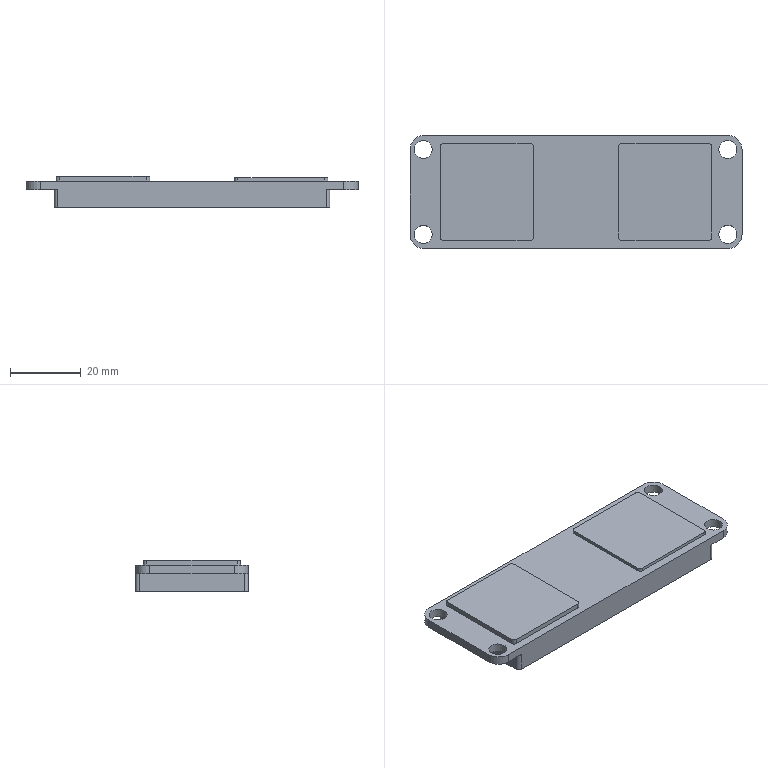CAM job | NX | 3-axis milling, drilling | part box 94 x 32 x 9 mm | stock box 94 x 32 x 9 mm
Tools:
number,name,description,diameter,corner_radius,flute_length,length,flutes
2,ER25-D10-20,Milling Tool-5 Parameters,10.0,0.0,20.0,20.0,2
3,ER25-D4-10,Milling Tool-5 Parameters,4.0,0.0,10.0,12.0,2
4,ER25-D1.5R0.3-23,Milling Tool-5 Parameters,1.5,0.3,5.0,5.0,2
10,ER25-D10-30_G,Milling Tool-5 Parameters,10.0,0.0,20.0,30.0,2
11,ER25-D4-23_G,Milling Tool-5 Parameters,4.0,0.0,10.0,23.0,2
1,D50-120,Milling Tool-5 Parameters,50.0,0.0,5.0,120.0,2
8,M3_D2.6,Drilling Tool,2.6,0.0,20.0,25.0,2
9,M3,Drilling Tool,2.6,0.0,15.0,20.0,2
7,DR_D5.1,Drilling Tool,5.1,0.0,10.0,50.0,2
5,Φ6倒角刀,Chamfer Mill,6.0,0.0,20.0,30.0,2
6,Φ3倒角刀,Chamfer Mill,3.0,0.0,10.0,10.0,2
Operations:
program,operation,operation_type,tool,method,geometry_group,spindle_rpm,surface_speed,feed_per_tooth,feed_cut,feed_plunge,cut_length_mm,path_length_mm,cut_time_min,machine_time_min
工件图层200层,101,VolumeBased25DMillingOperation,D50-120,METHOD,MCS_MILL,3000.0,471.0,0.1667,1000.0,100.0,179.0,278.0,0.179,0.1889
工件图层200层,102,PlanarMilling,ER25-D10-20,METHOD,MCS_MILL,6500.0,204.0,0.3462,4500.0,100.0,2909.584,3079.122,0.6466,0.6737
工件图层200层,PLANAR_PROFILE,PlanarMilling,ER25-D10-20,METHOD,MCS_MILL,6500.0,204.0,0.3462,4500.0,100.0,645.584,933.587,0.1435,0.1853
工件图层200层,103,PlanarMilling,ER25-D4-10,METHOD,MCS_MILL,6500.0,81.0,0.1923,2500.0,100.0,5110.233,5215.033,2.044,2.061
工件图层200层,104,PlanarMilling,ER25-D1.5R0.3-23,METHOD,MCS_MILL,6500.0,30.0,0.0923,1200.0,100.0,3417.434,3518.234,2.848,2.864
工件图层200层,SPOT_FACING,Operation,Φ6倒角刀,METHOD,MCS_MILL,2000.0,188.0,0.0125,100.0,100.0,15.0,261.648,0.15,0.1747
工件图层200层,105,Operation,Φ6倒角刀,METHOD,MCS_MILL,2000.0,188.0,0.0125,100.0,100.0,14.6,276.697,0.146,0.1722
工件图层200层,PLANAR_MILL_1_2,PlanarMilling,Φ6倒角刀,METHOD,MCS_MILL,5000.0,94.0,0.1,1000.0,100.0,239.176,342.176,0.2392,0.2558
工件图层200层,PLANAR_MILL_1_2_COPY,PlanarMilling,Φ6倒角刀,METHOD,MCS_MILL,5000.0,94.0,0.1,1000.0,100.0,244.733,347.733,0.2447,0.2613
工件图层200层,106,PlanarMilling,Φ3倒角刀,METHOD,MCS_MILL,5000.0,94.0,0.1,1000.0,100.0,95.688,395.588,0.0957,0.139
工件图层200层,107,Operation,DR_D5.1,METHOD,MCS_MILL,2000.0,188.0,0.0125,100.0,100.0,29.889,307.275,0.2989,0.3266
工件图层200层,108,Operation,M3_D2.6,METHOD,MCS_MILL,2000.0,188.0,0.0125,100.0,100.0,43.503,318.655,0.435,0.4625
工件图层200层,109,Operation,M3,METHOD,MCS_MILL,300.0,2.0,0.25,150.0,100.0,34.503,300.655,0.23,0.2566
工件图层200层,1010,PlanarMilling,ER25-D10-30_G,METHOD,MCS_MILL,5000.0,157.0,0.1,1000.0,100.0,582.313,701.313,0.5823,0.6015
工件图层200层,PLANAR_PROFILE_COPY,PlanarMilling,ER25-D10-30_G,METHOD,MCS_MILL,5000.0,157.0,0.1,1000.0,100.0,127.295,415.698,0.1273,0.1696
工件图层200层,PLANAR_PROFILE_COPY_COPY,PlanarMilling,ER25-D10-30_G,METHOD,MCS_MILL,5000.0,157.0,0.1,1000.0,100.0,127.232,415.635,0.1272,0.1695
工件图层200层,1011,PlanarMilling,ER25-D4-23_G,METHOD,MCS_MILL,5000.0,62.0,0.05,500.0,100.0,243.276,352.476,0.4866,0.5041
工件图层200层,1012,PlanarMilling,ER25-D1.5R0.3-23,METHOD,MCS_MILL,5000.0,62.0,0.05,500.0,100.0,539.151,640.351,1.078,1.095
工件图层200层,PLANAR_MILL_1_1_COPY_COPY_COPY,PlanarMilling,ER25-D1.5R0.3-23,METHOD,MCS_MILL,5000.0,62.0,0.05,500.0,100.0,531.35,632.55,1.063,1.079
PROGRAM_1,101_COPY,VolumeBased25DMillingOperation,D50-120,METHOD,MCS,3000.0,471.0,0.5,3000.0,100.0,1365.0,3174.6,0.455,0.636
PROGRAM_1,1013,FaceMilling,ER25-D10-20,METHOD,MCS,5000.0,157.0,0.2,2000.0,100.0,431.617,780.517,0.2158,0.2507
PROGRAM_1,1013_COPY,FaceMilling,ER25-D10-30_G,METHOD,MCS,5000.0,157.0,0.1,1000.0,100.0,369.0,611.286,0.369,0.3932
PROGRAM_1,1014,FaceMilling,ER25-D10-30_G,METHOD,MCS,5000.0,157.0,0.1,1000.0,100.0,491.763,894.655,0.4918,0.5321
PROGRAM_1,PLANAR_MILL_1_3,PlanarMilling,ER25-D10-30_G,METHOD,MCS,5000.0,157.0,0.1,1000.0,100.0,302.448,486.592,0.3024,0.3326
PROGRAM_1,1015,PlanarMilling,Φ3倒角刀,METHOD,MCS,5000.0,47.0,0.1,1000.0,100.0,231.789,402.967,0.2318,0.2598
PROGRAM_1,PLANAR_MILL_1_3_COPY_COPY,PlanarMilling,Φ3倒角刀,METHOD,MCS,5000.0,47.0,0.1,1000.0,100.0,256.315,359.115,0.2563,0.2729
PROGRAM_1,PLANAR_MILL_1_3_COPY_COPY_COPY,PlanarMilling,Φ3倒角刀,METHOD,MCS,5000.0,47.0,0.1,1000.0,100.0,64.551,609.889,0.0646,0.1442